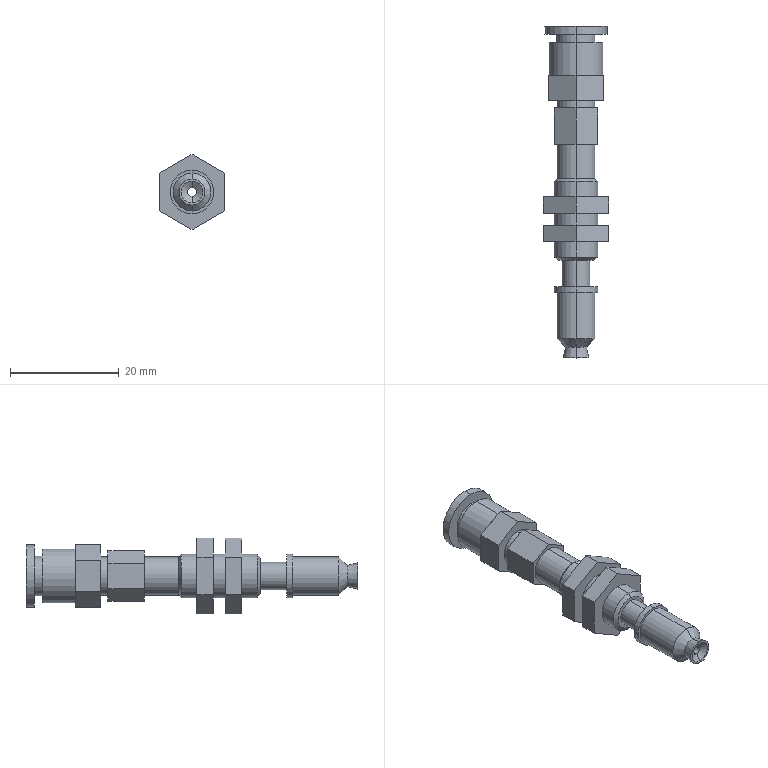Part | STEP file | Suction nozzle ZPT04UNJ6-06-A8 | 1 solid | 77 faces | box 12 x 61 x 13.856 mm | volume 3226 mm3 | plane 41 | cylinder 26 | cone 10 | commonest cylinder face diameters 8 x8 7 x6 1.6 x2 5 x2 6 x2 7.2 x2